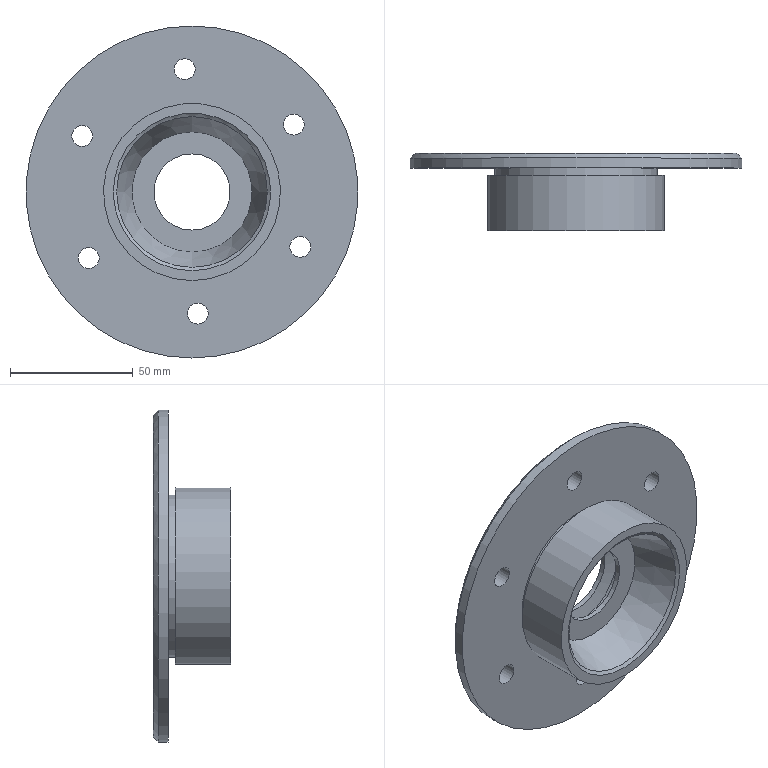Part | NX | features BREP 1, DATUM_CSYS 1 | 1 solid | 24 faces | box 135 x 31.5 x 135 mm | volume 118525 mm3 | cylinder 12 | plane 6 | cone 6 | commonest cylinder face diameters 8.5 x6 31 x2 43 x1 66 x1 72 x1 135 x1
STEP:
#1=CARTESIAN_POINT('',(160.,681.,-36.));
#2=VERTEX_POINT('',#1);
#3=CARTESIAN_POINT('',(160.,681.,0.));
#4=DIRECTION('',(0.,-1.,0.));
#5=DIRECTION('',(0.,0.,-1.));
#6=AXIS2_PLACEMENT_3D('',#3,#4,#5);
#7=CIRCLE('',#6,36.);
#8=EDGE_CURVE('',#2,#2,#7,.T.);
#9=ORIENTED_EDGE('',*,*,#8,.T.);
#10=EDGE_LOOP('',(#9));
#11=FACE_BOUND('',#10,.T.);
#12=CARTESIAN_POINT('',(160.,658.5,-36.));
#13=VERTEX_POINT('',#12);
#14=CARTESIAN_POINT('',(160.,658.5,0.));
#15=DIRECTION('',(0.,-1.,0.));
#16=DIRECTION('',(0.,0.,-1.));
#17=AXIS2_PLACEMENT_3D('',#14,#15,#16);
#18=CIRCLE('',#17,36.);
#19=EDGE_CURVE('',#13,#13,#18,.T.);
#20=ORIENTED_EDGE('',*,*,#19,.F.);
#21=EDGE_LOOP('',(#20));
#22=FACE_BOUND('',#21,.T.);
#23=CARTESIAN_POINT('',(160.,658.5,0.));
#24=DIRECTION('',(0.,-1.,0.));
#25=DIRECTION('',(0.,0.,-1.));
#26=AXIS2_PLACEMENT_3D('',#23,#24,#25);
#27=CYLINDRICAL_SURFACE('',#26,36.);
#28=ADVANCED_FACE('',(#11,#22),#27,.T.);
#29=CARTESIAN_POINT('',(160.,681.,-33.));
#30=VERTEX_POINT('',#29);
#31=CARTESIAN_POINT('',(160.,681.,0.));
#32=DIRECTION('',(0.,-1.,0.));
#33=DIRECTION('',(0.,0.,-1.));
#34=AXIS2_PLACEMENT_3D('',#31,#32,#33);
#35=CIRCLE('',#34,33.);
#36=EDGE_CURVE('',#30,#30,#35,.T.);
#37=ORIENTED_EDGE('',*,*,#36,.T.);
#38=EDGE_LOOP('',(#37));
#39=FACE_BOUND('',#38,.T.);
#40=ORIENTED_EDGE('',*,*,#8,.F.);
#41=EDGE_LOOP('',(#40));
#42=FACE_BOUND('',#41,.T.);
#43=CARTESIAN_POINT('',(196.,681.,0.));
#44=DIRECTION('',(0.,1.,0.));
#45=DIRECTION('',(0.,0.,1.));
#46=AXIS2_PLACEMENT_3D('',#43,#44,#45);
#47=PLANE('',#46);
#48=ADVANCED_FACE('',(#39,#42),#47,.T.);
#49=CARTESIAN_POINT('',(160.,684.,-33.));
#50=VERTEX_POINT('',#49);
#51=CARTESIAN_POINT('',(160.,684.,0.));
#52=DIRECTION('',(0.,-1.,0.));
#53=DIRECTION('',(0.,0.,-1.));
#54=AXIS2_PLACEMENT_3D('',#51,#52,#53);
#55=CIRCLE('',#54,33.);
#56=EDGE_CURVE('',#50,#50,#55,.T.);
#57=ORIENTED_EDGE('',*,*,#56,.T.);
#58=EDGE_LOOP('',(#57));
#59=FACE_BOUND('',#58,.T.);
#60=ORIENTED_EDGE('',*,*,#36,.F.);
#61=EDGE_LOOP('',(#60));
#62=FACE_BOUND('',#61,.T.);
#63=CARTESIAN_POINT('',(160.,658.5,0.));
#64=DIRECTION('',(0.,-1.,0.));
#65=DIRECTION('',(0.,0.,-1.));
#66=AXIS2_PLACEMENT_3D('',#63,#64,#65);
#67=CYLINDRICAL_SURFACE('',#66,33.);
#68=ADVANCED_FACE('',(#59,#62),#67,.T.);
#69=CARTESIAN_POINT('',(118.012,684.,-31.136));
#70=VERTEX_POINT('',#69);
#71=CARTESIAN_POINT('',(118.012,684.,-26.886));
#72=DIRECTION('',(0.,-1.,0.));
#73=DIRECTION('',(0.,0.,-1.));
#74=AXIS2_PLACEMENT_3D('',#71,#72,#73);
#75=CIRCLE('',#74,4.25);
#76=EDGE_CURVE('',#70,#70,#75,.F.);
#77=ORIENTED_EDGE('',*,*,#76,.T.);
#78=EDGE_LOOP('',(#77));
#79=FACE_BOUND('',#78,.T.);
#80=CARTESIAN_POINT('',(157.05,684.,45.663));
#81=VERTEX_POINT('',#80);
#82=CARTESIAN_POINT('',(157.05,684.,49.913));
#83=DIRECTION('',(0.,-1.,0.));
#84=DIRECTION('',(0.,0.,-1.));
#85=AXIS2_PLACEMENT_3D('',#82,#83,#84);
#86=CIRCLE('',#85,4.25);
#87=EDGE_CURVE('',#81,#81,#86,.F.);
#88=ORIENTED_EDGE('',*,*,#87,.T.);
#89=EDGE_LOOP('',(#88));
#90=FACE_BOUND('',#89,.T.);
#91=CARTESIAN_POINT('',(162.352,684.,-53.675));
#92=VERTEX_POINT('',#91);
#93=CARTESIAN_POINT('',(162.352,684.,-49.425));
#94=DIRECTION('',(0.,-1.,0.));
#95=DIRECTION('',(0.,0.,-1.));
#96=AXIS2_PLACEMENT_3D('',#93,#94,#95);
#97=CIRCLE('',#96,4.25);
#98=EDGE_CURVE('',#92,#92,#97,.F.);
#99=ORIENTED_EDGE('',*,*,#98,.T.);
#100=EDGE_LOOP('',(#99));
#101=FACE_BOUND('',#100,.T.);
#102=CARTESIAN_POINT('',(201.39,684.,23.124));
#103=VERTEX_POINT('',#102);
#104=CARTESIAN_POINT('',(201.39,684.,27.374));
#105=DIRECTION('',(0.,-1.,0.));
#106=DIRECTION('',(0.,0.,-1.));
#107=AXIS2_PLACEMENT_3D('',#104,#105,#106);
#108=CIRCLE('',#107,4.25);
#109=EDGE_CURVE('',#103,#103,#108,.F.);
#110=ORIENTED_EDGE('',*,*,#109,.T.);
#111=EDGE_LOOP('',(#110));
#112=FACE_BOUND('',#111,.T.);
#113=CARTESIAN_POINT('',(115.361,684.,18.533));
#114=VERTEX_POINT('',#113);
#115=CARTESIAN_POINT('',(115.361,684.,22.783));
#116=DIRECTION('',(0.,-1.,0.));
#117=DIRECTION('',(0.,0.,-1.));
#118=AXIS2_PLACEMENT_3D('',#115,#116,#117);
#119=CIRCLE('',#118,4.25);
#120=EDGE_CURVE('',#114,#114,#119,.F.);
#121=ORIENTED_EDGE('',*,*,#120,.T.);
#122=EDGE_LOOP('',(#121));
#123=FACE_BOUND('',#122,.T.);
#124=CARTESIAN_POINT('',(204.041,684.,-26.545));
#125=VERTEX_POINT('',#124);
#126=CARTESIAN_POINT('',(204.041,684.,-22.295));
#127=DIRECTION('',(0.,-1.,0.));
#128=DIRECTION('',(0.,0.,-1.));
#129=AXIS2_PLACEMENT_3D('',#126,#127,#128);
#130=CIRCLE('',#129,4.25);
#131=EDGE_CURVE('',#125,#125,#130,.F.);
#132=ORIENTED_EDGE('',*,*,#131,.T.);
#133=EDGE_LOOP('',(#132));
#134=FACE_BOUND('',#133,.T.);
#135=CARTESIAN_POINT('',(160.,684.,-67.5));
#136=VERTEX_POINT('',#135);
#137=CARTESIAN_POINT('',(160.,684.,0.));
#138=DIRECTION('',(0.,-1.,0.));
#139=DIRECTION('',(0.,0.,-1.));
#140=AXIS2_PLACEMENT_3D('',#137,#138,#139);
#141=CIRCLE('',#140,67.5);
#142=EDGE_CURVE('',#136,#136,#141,.T.);
#143=ORIENTED_EDGE('',*,*,#142,.T.);
#144=EDGE_LOOP('',(#143));
#145=FACE_BOUND('',#144,.T.);
#146=ORIENTED_EDGE('',*,*,#56,.F.);
#147=EDGE_LOOP('',(#146));
#148=FACE_BOUND('',#147,.T.);
#149=CARTESIAN_POINT('',(196.,684.,0.));
#150=DIRECTION('',(0.,-1.,0.));
#151=DIRECTION('',(0.,0.,-1.));
#152=AXIS2_PLACEMENT_3D('',#149,#150,#151);
#153=PLANE('',#152);
#154=ADVANCED_FACE('',(#79,#90,#101,#112,#123,#134,#145,#148),#153,.T.);
#155=CARTESIAN_POINT('',(160.,688.,-67.5));
#156=VERTEX_POINT('',#155);
#157=CARTESIAN_POINT('',(160.,688.,0.));
#158=DIRECTION('',(0.,-1.,0.));
#159=DIRECTION('',(0.,0.,-1.));
#160=AXIS2_PLACEMENT_3D('',#157,#158,#159);
#161=CIRCLE('',#160,67.5);
#162=EDGE_CURVE('',#156,#156,#161,.T.);
#163=ORIENTED_EDGE('',*,*,#162,.T.);
#164=EDGE_LOOP('',(#163));
#165=FACE_BOUND('',#164,.T.);
#166=ORIENTED_EDGE('',*,*,#142,.F.);
#167=EDGE_LOOP('',(#166));
#168=FACE_BOUND('',#167,.T.);
#169=CARTESIAN_POINT('',(160.,658.5,0.));
#170=DIRECTION('',(0.,-1.,0.));
#171=DIRECTION('',(0.,0.,-1.));
#172=AXIS2_PLACEMENT_3D('',#169,#170,#171);
#173=CYLINDRICAL_SURFACE('',#172,67.5);
#174=ADVANCED_FACE('',(#165,#168),#173,.T.);
#175=CARTESIAN_POINT('',(160.,690.,-65.5));
#176=VERTEX_POINT('',#175);
#177=CARTESIAN_POINT('',(160.,690.,0.));
#178=DIRECTION('',(0.,-1.,0.));
#179=DIRECTION('',(0.,0.,-1.));
#180=AXIS2_PLACEMENT_3D('',#177,#178,#179);
#181=CIRCLE('',#180,65.5);
#182=EDGE_CURVE('',#176,#176,#181,.T.);
#183=ORIENTED_EDGE('',*,*,#182,.T.);
#184=EDGE_LOOP('',(#183));
#185=FACE_BOUND('',#184,.T.);
#186=ORIENTED_EDGE('',*,*,#162,.F.);
#187=EDGE_LOOP('',(#186));
#188=FACE_BOUND('',#187,.T.);
#189=CARTESIAN_POINT('',(160.,688.,0.));
#190=DIRECTION('',(0.,-1.,0.));
#191=DIRECTION('',(0.,0.,-1.));
#192=AXIS2_PLACEMENT_3D('',#189,#190,#191);
#193=CONICAL_SURFACE('',#192,67.5,0.7854);
#194=ADVANCED_FACE('',(#185,#188),#193,.T.);
#195=CARTESIAN_POINT('',(118.012,690.,-22.636));
#196=VERTEX_POINT('',#195);
#197=CARTESIAN_POINT('',(118.012,690.,-26.886));
#198=DIRECTION('',(0.,1.,0.));
#199=DIRECTION('',(0.,0.,1.));
#200=AXIS2_PLACEMENT_3D('',#197,#198,#199);
#201=CIRCLE('',#200,4.25);
#202=EDGE_CURVE('',#196,#196,#201,.F.);
#203=ORIENTED_EDGE('',*,*,#202,.T.);
#204=EDGE_LOOP('',(#203));
#205=FACE_BOUND('',#204,.T.);
#206=CARTESIAN_POINT('',(157.05,690.,54.163));
#207=VERTEX_POINT('',#206);
#208=CARTESIAN_POINT('',(157.05,690.,49.913));
#209=DIRECTION('',(0.,1.,0.));
#210=DIRECTION('',(0.,0.,1.));
#211=AXIS2_PLACEMENT_3D('',#208,#209,#210);
#212=CIRCLE('',#211,4.25);
#213=EDGE_CURVE('',#207,#207,#212,.F.);
#214=ORIENTED_EDGE('',*,*,#213,.T.);
#215=EDGE_LOOP('',(#214));
#216=FACE_BOUND('',#215,.T.);
#217=CARTESIAN_POINT('',(162.352,690.,-45.175));
#218=VERTEX_POINT('',#217);
#219=CARTESIAN_POINT('',(162.352,690.,-49.425));
#220=DIRECTION('',(0.,1.,0.));
#221=DIRECTION('',(0.,0.,1.));
#222=AXIS2_PLACEMENT_3D('',#219,#220,#221);
#223=CIRCLE('',#222,4.25);
#224=EDGE_CURVE('',#218,#218,#223,.F.);
#225=ORIENTED_EDGE('',*,*,#224,.T.);
#226=EDGE_LOOP('',(#225));
#227=FACE_BOUND('',#226,.T.);
#228=CARTESIAN_POINT('',(201.39,690.,31.624));
#229=VERTEX_POINT('',#228);
#230=CARTESIAN_POINT('',(201.39,690.,27.374));
#231=DIRECTION('',(0.,1.,0.));
#232=DIRECTION('',(0.,0.,1.));
#233=AXIS2_PLACEMENT_3D('',#230,#231,#232);
#234=CIRCLE('',#233,4.25);
#235=EDGE_CURVE('',#229,#229,#234,.F.);
#236=ORIENTED_EDGE('',*,*,#235,.T.);
#237=EDGE_LOOP('',(#236));
#238=FACE_BOUND('',#237,.T.);
#239=CARTESIAN_POINT('',(115.361,690.,27.033));
#240=VERTEX_POINT('',#239);
#241=CARTESIAN_POINT('',(115.361,690.,22.783));
#242=DIRECTION('',(0.,1.,0.));
#243=DIRECTION('',(0.,0.,1.));
#244=AXIS2_PLACEMENT_3D('',#241,#242,#243);
#245=CIRCLE('',#244,4.25);
#246=EDGE_CURVE('',#240,#240,#245,.F.);
#247=ORIENTED_EDGE('',*,*,#246,.T.);
#248=EDGE_LOOP('',(#247));
#249=FACE_BOUND('',#248,.T.);
#250=CARTESIAN_POINT('',(204.041,690.,-18.045));
#251=VERTEX_POINT('',#250);
#252=CARTESIAN_POINT('',(204.041,690.,-22.295));
#253=DIRECTION('',(0.,1.,0.));
#254=DIRECTION('',(0.,0.,1.));
#255=AXIS2_PLACEMENT_3D('',#252,#253,#254);
#256=CIRCLE('',#255,4.25);
#257=EDGE_CURVE('',#251,#251,#256,.F.);
#258=ORIENTED_EDGE('',*,*,#257,.T.);
#259=EDGE_LOOP('',(#258));
#260=FACE_BOUND('',#259,.T.);
#261=CARTESIAN_POINT('',(160.,690.,-35.5));
#262=VERTEX_POINT('',#261);
#263=CARTESIAN_POINT('',(160.,690.,0.));
#264=DIRECTION('',(0.,-1.,0.));
#265=DIRECTION('',(0.,0.,-1.));
#266=AXIS2_PLACEMENT_3D('',#263,#264,#265);
#267=CIRCLE('',#266,35.5);
#268=EDGE_CURVE('',#262,#262,#267,.T.);
#269=ORIENTED_EDGE('',*,*,#268,.T.);
#270=EDGE_LOOP('',(#269));
#271=FACE_BOUND('',#270,.T.);
#272=ORIENTED_EDGE('',*,*,#182,.F.);
#273=EDGE_LOOP('',(#272));
#274=FACE_BOUND('',#273,.T.);
#275=CARTESIAN_POINT('',(225.5,690.,0.));
#276=DIRECTION('',(0.,1.,0.));
#277=DIRECTION('',(0.,0.,1.));
#278=AXIS2_PLACEMENT_3D('',#275,#276,#277);
#279=PLANE('',#278);
#280=ADVANCED_FACE('',(#205,#216,#227,#238,#249,#260,#271,#274),#279,.T.);
#281=CARTESIAN_POINT('',(160.,687.,-32.5));
#282=VERTEX_POINT('',#281);
#283=CARTESIAN_POINT('',(160.,687.,0.));
#284=DIRECTION('',(0.,-1.,0.));
#285=DIRECTION('',(0.,0.,-1.));
#286=AXIS2_PLACEMENT_3D('',#283,#284,#285);
#287=CIRCLE('',#286,32.5);
#288=EDGE_CURVE('',#282,#282,#287,.T.);
#289=ORIENTED_EDGE('',*,*,#288,.T.);
#290=EDGE_LOOP('',(#289));
#291=FACE_BOUND('',#290,.T.);
#292=ORIENTED_EDGE('',*,*,#268,.F.);
#293=EDGE_LOOP('',(#292));
#294=FACE_BOUND('',#293,.T.);
#295=CARTESIAN_POINT('',(160.,690.,0.));
#296=DIRECTION('',(0.,1.,0.));
#297=DIRECTION('',(0.,0.,1.));
#298=AXIS2_PLACEMENT_3D('',#295,#296,#297);
#299=CONICAL_SURFACE('',#298,35.5,0.7854);
#300=ADVANCED_FACE('',(#291,#294),#299,.F.);
#301=CARTESIAN_POINT('',(160.,687.,-15.5));
#302=VERTEX_POINT('',#301);
#303=CARTESIAN_POINT('',(160.,687.,0.));
#304=DIRECTION('',(0.,-1.,0.));
#305=DIRECTION('',(0.,0.,-1.));
#306=AXIS2_PLACEMENT_3D('',#303,#304,#305);
#307=CIRCLE('',#306,15.5);
#308=EDGE_CURVE('',#302,#302,#307,.T.);
#309=ORIENTED_EDGE('',*,*,#308,.T.);
#310=EDGE_LOOP('',(#309));
#311=FACE_BOUND('',#310,.T.);
#312=ORIENTED_EDGE('',*,*,#288,.F.);
#313=EDGE_LOOP('',(#312));
#314=FACE_BOUND('',#313,.T.);
#315=CARTESIAN_POINT('',(192.5,687.,0.));
#316=DIRECTION('',(0.,1.,0.));
#317=DIRECTION('',(0.,0.,1.));
#318=AXIS2_PLACEMENT_3D('',#315,#316,#317);
#319=PLANE('',#318);
#320=ADVANCED_FACE('',(#311,#314),#319,.T.);
#321=CARTESIAN_POINT('',(160.,685.,-15.5));
#322=VERTEX_POINT('',#321);
#323=CARTESIAN_POINT('',(160.,685.,0.));
#324=DIRECTION('',(0.,-1.,0.));
#325=DIRECTION('',(0.,0.,-1.));
#326=AXIS2_PLACEMENT_3D('',#323,#324,#325);
#327=CIRCLE('',#326,15.5);
#328=EDGE_CURVE('',#322,#322,#327,.T.);
#329=ORIENTED_EDGE('',*,*,#328,.T.);
#330=EDGE_LOOP('',(#329));
#331=FACE_BOUND('',#330,.T.);
#332=ORIENTED_EDGE('',*,*,#308,.F.);
#333=EDGE_LOOP('',(#332));
#334=FACE_BOUND('',#333,.T.);
#335=CARTESIAN_POINT('',(160.,658.5,0.));
#336=DIRECTION('',(0.,-1.,0.));
#337=DIRECTION('',(0.,0.,-1.));
#338=AXIS2_PLACEMENT_3D('',#335,#336,#337);
#339=CYLINDRICAL_SURFACE('',#338,15.5);
#340=ADVANCED_FACE('',(#331,#334),#339,.F.);
#341=CARTESIAN_POINT('',(160.,683.95,-21.5));
#342=VERTEX_POINT('',#341);
#343=CARTESIAN_POINT('',(160.,683.95,0.));
#344=DIRECTION('',(0.,-1.,0.));
#345=DIRECTION('',(0.,0.,-1.));
#346=AXIS2_PLACEMENT_3D('',#343,#344,#345);
#347=CIRCLE('',#346,21.5);
#348=EDGE_CURVE('',#342,#342,#347,.T.);
#349=ORIENTED_EDGE('',*,*,#348,.T.);
#350=EDGE_LOOP('',(#349));
#351=FACE_BOUND('',#350,.T.);
#352=ORIENTED_EDGE('',*,*,#328,.F.);
#353=EDGE_LOOP('',(#352));
#354=FACE_BOUND('',#353,.T.);
#355=CARTESIAN_POINT('',(160.,685.,0.));
#356=DIRECTION('',(0.,-1.,0.));
#357=DIRECTION('',(0.,0.,-1.));
#358=AXIS2_PLACEMENT_3D('',#355,#356,#357);
#359=CONICAL_SURFACE('',#358,15.5,1.398);
#360=ADVANCED_FACE('',(#351,#354),#359,.F.);
#361=CARTESIAN_POINT('',(160.,679.55,-21.5));
#362=VERTEX_POINT('',#361);
#363=CARTESIAN_POINT('',(160.,679.55,0.));
#364=DIRECTION('',(0.,-1.,0.));
#365=DIRECTION('',(0.,0.,-1.));
#366=AXIS2_PLACEMENT_3D('',#363,#364,#365);
#367=CIRCLE('',#366,21.5);
#368=EDGE_CURVE('',#362,#362,#367,.T.);
#369=ORIENTED_EDGE('',*,*,#368,.T.);
#370=EDGE_LOOP('',(#369));
#371=FACE_BOUND('',#370,.T.);
#372=ORIENTED_EDGE('',*,*,#348,.F.);
#373=EDGE_LOOP('',(#372));
#374=FACE_BOUND('',#373,.T.);
#375=CARTESIAN_POINT('',(160.,658.5,0.));
#376=DIRECTION('',(0.,-1.,0.));
#377=DIRECTION('',(0.,0.,-1.));
#378=AXIS2_PLACEMENT_3D('',#375,#376,#377);
#379=CYLINDRICAL_SURFACE('',#378,21.5);
#380=ADVANCED_FACE('',(#371,#374),#379,.F.);
#381=CARTESIAN_POINT('',(160.,678.5,-15.5));
#382=VERTEX_POINT('',#381);
#383=CARTESIAN_POINT('',(160.,678.5,0.));
#384=DIRECTION('',(0.,-1.,0.));
#385=DIRECTION('',(0.,0.,-1.));
#386=AXIS2_PLACEMENT_3D('',#383,#384,#385);
#387=CIRCLE('',#386,15.5);
#388=EDGE_CURVE('',#382,#382,#387,.T.);
#389=ORIENTED_EDGE('',*,*,#388,.T.);
#390=EDGE_LOOP('',(#389));
#391=FACE_BOUND('',#390,.T.);
#392=ORIENTED_EDGE('',*,*,#368,.F.);
#393=EDGE_LOOP('',(#392));
#394=FACE_BOUND('',#393,.T.);
#395=CARTESIAN_POINT('',(160.,679.55,0.));
#396=DIRECTION('',(0.,1.,0.));
#397=DIRECTION('',(0.,0.,1.));
#398=AXIS2_PLACEMENT_3D('',#395,#396,#397);
#399=CONICAL_SURFACE('',#398,21.5,1.398);
#400=ADVANCED_FACE('',(#391,#394),#399,.F.);
#401=CARTESIAN_POINT('',(160.,676.5,-15.5));
#402=VERTEX_POINT('',#401);
#403=CARTESIAN_POINT('',(160.,676.5,0.));
#404=DIRECTION('',(0.,-1.,0.));
#405=DIRECTION('',(0.,0.,-1.));
#406=AXIS2_PLACEMENT_3D('',#403,#404,#405);
#407=CIRCLE('',#406,15.5);
#408=EDGE_CURVE('',#402,#402,#407,.T.);
#409=ORIENTED_EDGE('',*,*,#408,.T.);
#410=EDGE_LOOP('',(#409));
#411=FACE_BOUND('',#410,.T.);
#412=ORIENTED_EDGE('',*,*,#388,.F.);
#413=EDGE_LOOP('',(#412));
#414=FACE_BOUND('',#413,.T.);
#415=CARTESIAN_POINT('',(160.,658.5,0.));
#416=DIRECTION('',(0.,-1.,0.));
#417=DIRECTION('',(0.,0.,-1.));
#418=AXIS2_PLACEMENT_3D('',#415,#416,#417);
#419=CYLINDRICAL_SURFACE('',#418,15.5);
#420=ADVANCED_FACE('',(#411,#414),#419,.F.);
#421=CARTESIAN_POINT('',(160.,676.5,-24.449));
#422=VERTEX_POINT('',#421);
#423=CARTESIAN_POINT('',(160.,676.5,0.));
#424=DIRECTION('',(0.,-1.,0.));
#425=DIRECTION('',(0.,0.,-1.));
#426=AXIS2_PLACEMENT_3D('',#423,#424,#425);
#427=CIRCLE('',#426,24.449);
#428=EDGE_CURVE('',#422,#422,#427,.T.);
#429=ORIENTED_EDGE('',*,*,#428,.T.);
#430=EDGE_LOOP('',(#429));
#431=FACE_BOUND('',#430,.T.);
#432=ORIENTED_EDGE('',*,*,#408,.F.);
#433=EDGE_LOOP('',(#432));
#434=FACE_BOUND('',#433,.T.);
#435=CARTESIAN_POINT('',(175.5,676.5,0.));
#436=DIRECTION('',(0.,-1.,0.));
#437=DIRECTION('',(0.,0.,-1.));
#438=AXIS2_PLACEMENT_3D('',#435,#436,#437);
#439=PLANE('',#438);
#440=ADVANCED_FACE('',(#431,#434),#439,.T.);
#441=CARTESIAN_POINT('',(160.,659.44,-30.658));
#442=VERTEX_POINT('',#441);
#443=CARTESIAN_POINT('',(160.,659.44,0.));
#444=DIRECTION('',(0.,-1.,0.));
#445=DIRECTION('',(0.,0.,-1.));
#446=AXIS2_PLACEMENT_3D('',#443,#444,#445);
#447=CIRCLE('',#446,30.658);
#448=EDGE_CURVE('',#442,#442,#447,.T.);
#449=ORIENTED_EDGE('',*,*,#448,.T.);
#450=EDGE_LOOP('',(#449));
#451=FACE_BOUND('',#450,.T.);
#452=ORIENTED_EDGE('',*,*,#428,.F.);
#453=EDGE_LOOP('',(#452));
#454=FACE_BOUND('',#453,.T.);
#455=CARTESIAN_POINT('',(160.,676.5,0.));
#456=DIRECTION('',(0.,-1.,0.));
#457=DIRECTION('',(0.,0.,-1.));
#458=AXIS2_PLACEMENT_3D('',#455,#456,#457);
#459=CONICAL_SURFACE('',#458,24.449,0.3491);
#460=ADVANCED_FACE('',(#451,#454),#459,.F.);
#461=CARTESIAN_POINT('',(160.,658.5,-32.));
#462=VERTEX_POINT('',#461);
#463=CARTESIAN_POINT('',(160.,658.5,0.));
#464=DIRECTION('',(0.,-1.,0.));
#465=DIRECTION('',(0.,0.,-1.));
#466=AXIS2_PLACEMENT_3D('',#463,#464,#465);
#467=CIRCLE('',#466,32.);
#468=EDGE_CURVE('',#462,#462,#467,.T.);
#469=ORIENTED_EDGE('',*,*,#468,.T.);
#470=EDGE_LOOP('',(#469));
#471=FACE_BOUND('',#470,.T.);
#472=ORIENTED_EDGE('',*,*,#448,.F.);
#473=EDGE_LOOP('',(#472));
#474=FACE_BOUND('',#473,.T.);
#475=CARTESIAN_POINT('',(160.,659.44,0.));
#476=DIRECTION('',(0.,-1.,0.));
#477=DIRECTION('',(0.,0.,-1.));
#478=AXIS2_PLACEMENT_3D('',#475,#476,#477);
#479=CONICAL_SURFACE('',#478,30.658,0.9599);
#480=ADVANCED_FACE('',(#471,#474),#479,.F.);
#481=ORIENTED_EDGE('',*,*,#19,.T.);
#482=EDGE_LOOP('',(#481));
#483=FACE_BOUND('',#482,.T.);
#484=ORIENTED_EDGE('',*,*,#468,.F.);
#485=EDGE_LOOP('',(#484));
#486=FACE_BOUND('',#485,.T.);
#487=CARTESIAN_POINT('',(192.,658.5,0.));
#488=DIRECTION('',(0.,-1.,0.));
#489=DIRECTION('',(0.,0.,-1.));
#490=AXIS2_PLACEMENT_3D('',#487,#488,#489);
#491=PLANE('',#490);
#492=ADVANCED_FACE('',(#483,#486),#491,.T.);
#493=ORIENTED_EDGE('',*,*,#131,.F.);
#494=EDGE_LOOP('',(#493));
#495=FACE_BOUND('',#494,.T.);
#496=ORIENTED_EDGE('',*,*,#257,.F.);
#497=EDGE_LOOP('',(#496));
#498=FACE_BOUND('',#497,.T.);
#499=CARTESIAN_POINT('',(204.041,740.,-22.295));
#500=DIRECTION('',(0.,-1.,0.));
#501=DIRECTION('',(0.,0.,-1.));
#502=AXIS2_PLACEMENT_3D('',#499,#500,#501);
#503=CYLINDRICAL_SURFACE('',#502,4.25);
#504=ADVANCED_FACE('',(#495,#498),#503,.F.);
#505=ORIENTED_EDGE('',*,*,#120,.F.);
#506=EDGE_LOOP('',(#505));
#507=FACE_BOUND('',#506,.T.);
#508=ORIENTED_EDGE('',*,*,#246,.F.);
#509=EDGE_LOOP('',(#508));
#510=FACE_BOUND('',#509,.T.);
#511=CARTESIAN_POINT('',(115.361,740.,22.783));
#512=DIRECTION('',(0.,-1.,0.));
#513=DIRECTION('',(0.,0.,-1.));
#514=AXIS2_PLACEMENT_3D('',#511,#512,#513);
#515=CYLINDRICAL_SURFACE('',#514,4.25);
#516=ADVANCED_FACE('',(#507,#510),#515,.F.);
#517=ORIENTED_EDGE('',*,*,#109,.F.);
#518=EDGE_LOOP('',(#517));
#519=FACE_BOUND('',#518,.T.);
#520=ORIENTED_EDGE('',*,*,#235,.F.);
#521=EDGE_LOOP('',(#520));
#522=FACE_BOUND('',#521,.T.);
#523=CARTESIAN_POINT('',(201.39,740.,27.374));
#524=DIRECTION('',(0.,-1.,0.));
#525=DIRECTION('',(0.,0.,-1.));
#526=AXIS2_PLACEMENT_3D('',#523,#524,#525);
#527=CYLINDRICAL_SURFACE('',#526,4.25);
#528=ADVANCED_FACE('',(#519,#522),#527,.F.);
#529=ORIENTED_EDGE('',*,*,#98,.F.);
#530=EDGE_LOOP('',(#529));
#531=FACE_BOUND('',#530,.T.);
#532=ORIENTED_EDGE('',*,*,#224,.F.);
#533=EDGE_LOOP('',(#532));
#534=FACE_BOUND('',#533,.T.);
#535=CARTESIAN_POINT('',(162.352,740.,-49.425));
#536=DIRECTION('',(0.,-1.,0.));
#537=DIRECTION('',(0.,0.,-1.));
#538=AXIS2_PLACEMENT_3D('',#535,#536,#537);
#539=CYLINDRICAL_SURFACE('',#538,4.25);
#540=ADVANCED_FACE('',(#531,#534),#539,.F.);
#541=ORIENTED_EDGE('',*,*,#87,.F.);
#542=EDGE_LOOP('',(#541));
#543=FACE_BOUND('',#542,.T.);
#544=ORIENTED_EDGE('',*,*,#213,.F.);
#545=EDGE_LOOP('',(#544));
#546=FACE_BOUND('',#545,.T.);
#547=CARTESIAN_POINT('',(157.05,740.,49.913));
#548=DIRECTION('',(0.,-1.,0.));
#549=DIRECTION('',(0.,0.,-1.));
#550=AXIS2_PLACEMENT_3D('',#547,#548,#549);
#551=CYLINDRICAL_SURFACE('',#550,4.25);
#552=ADVANCED_FACE('',(#543,#546),#551,.F.);
#553=ORIENTED_EDGE('',*,*,#76,.F.);
#554=EDGE_LOOP('',(#553));
#555=FACE_BOUND('',#554,.T.);
#556=ORIENTED_EDGE('',*,*,#202,.F.);
#557=EDGE_LOOP('',(#556));
#558=FACE_BOUND('',#557,.T.);
#559=CARTESIAN_POINT('',(118.012,740.,-26.886));
#560=DIRECTION('',(0.,-1.,0.));
#561=DIRECTION('',(0.,0.,-1.));
#562=AXIS2_PLACEMENT_3D('',#559,#560,#561);
#563=CYLINDRICAL_SURFACE('',#562,4.25);
#564=ADVANCED_FACE('',(#555,#558),#563,.F.);
#565=CLOSED_SHELL('',(#28,#48,#68,#154,#174,#194,#280,#300,#320,#340,#360,#380,#400,#420,#440,#460,#480,#492,#504,#516,#528,#540,#552,#564));
#566=MANIFOLD_SOLID_BREP('',#565);
#567=(LENGTH_UNIT()NAMED_UNIT(*)SI_UNIT(.MILLI.,.METRE.));
#568=UNCERTAINTY_MEASURE_WITH_UNIT(LENGTH_MEASURE(0.00001),#567,'','');
#569=(NAMED_UNIT(*)PLANE_ANGLE_UNIT()SI_UNIT($,.RADIAN.));
#570=(NAMED_UNIT(*)SI_UNIT($,.STERADIAN.)SOLID_ANGLE_UNIT());
#571=(GEOMETRIC_REPRESENTATION_CONTEXT(3)GLOBAL_UNCERTAINTY_ASSIGNED_CONTEXT((#568))GLOBAL_UNIT_ASSIGNED_CONTEXT((#567,#569,#570))REPRESENTATION_CONTEXT('',''));
#572=ADVANCED_BREP_SHAPE_REPRESENTATION('',(#566),#571);